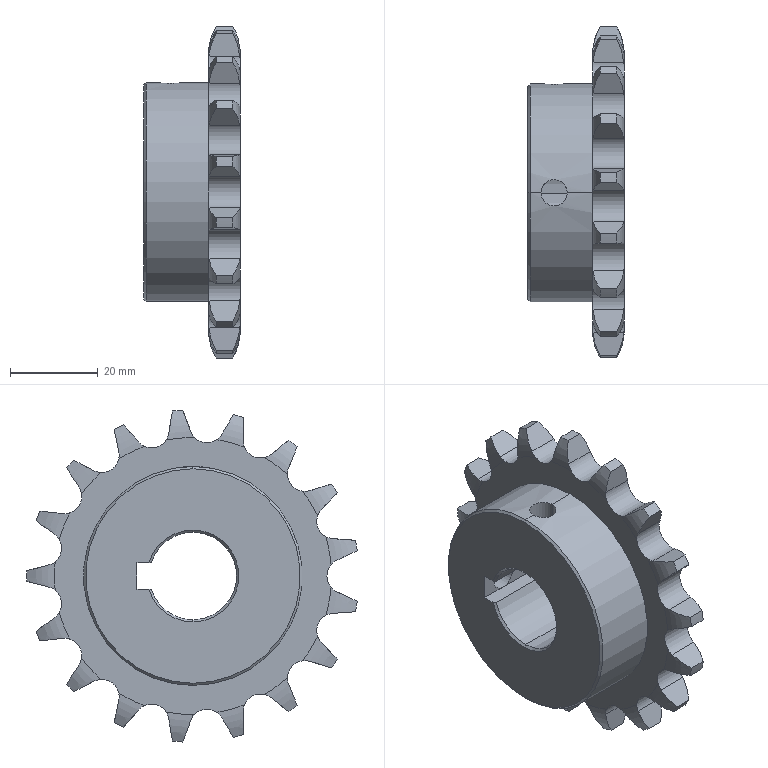Part | STEP file | J011-EBZ05-04-00-Part-1 | 1 solid | 128 faces | box 22 x 75.554 x 75.859 mm | volume 46001 mm3 | cylinder 43 | plane 41 | torus 36 | cone 8 | commonest cylinder face diameters 7.92 x17 76 x17 6 x4 20 x3 50 x2